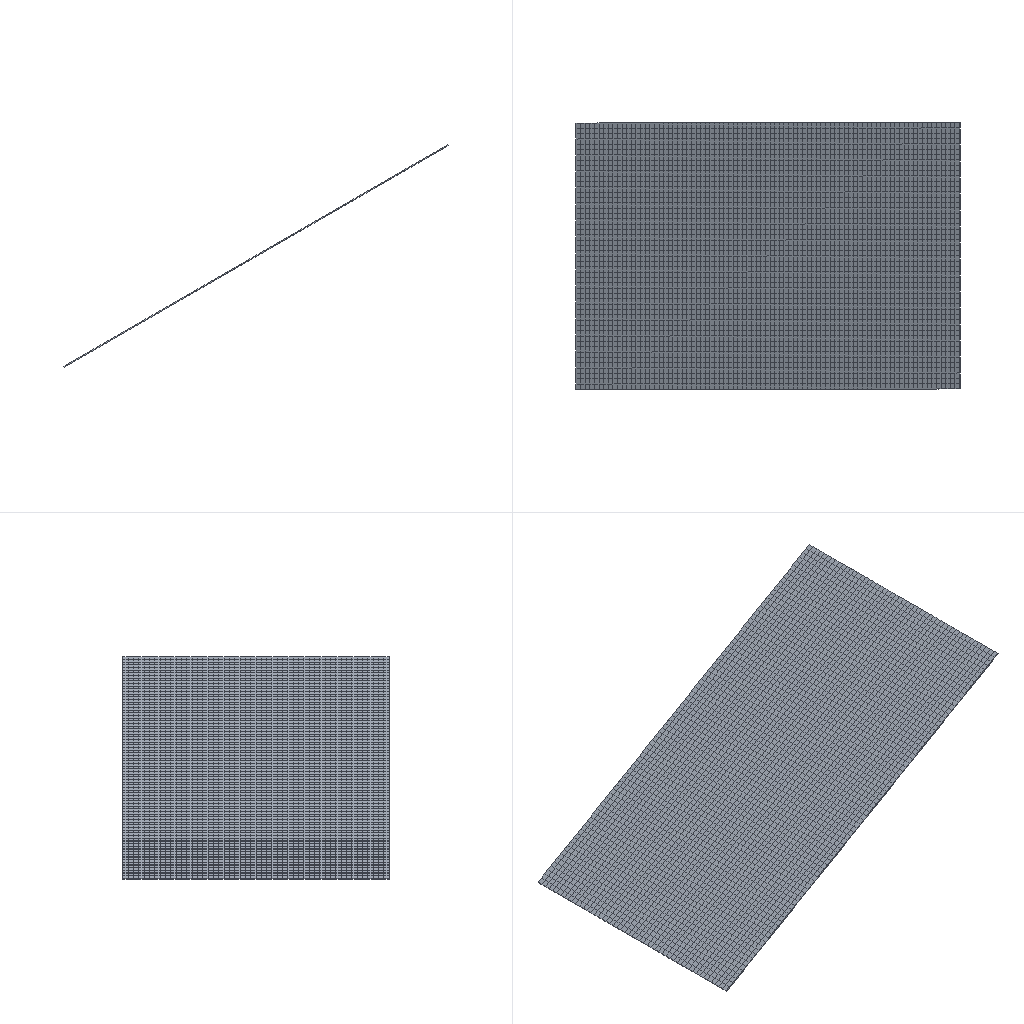Simulation study | abaqus
Set-up summary:
category,name,step,type,value,unit,region
solver,abaqus
solver,version,,,Abaqus/Standard 2020
units,not stated in the deck,,not stated
analysis,deck,,static,static
load_step,Step-1,Step-1,static
load_step,requested,,,1
mesh,nodes,,,21420
mesh,elements,,,16600
element_type,C3D8R,,solid,16600
load,load commands in deck,,count,1
bc,support commands in deck,,count,1
material,LAY1,,in results
material,LAY2,,in results
material,LAY4,,in results
check,setup vs results,,match,"per instance, exact: element labels, types and connectivity; labels of the nodes the elements use; coordinates of those nodes at SINGLE_PRECISION in 1 of 1 instance(s)"
Abaqus input file, long lists of numbers shortened:
*Heading
** Job name: Job-1 Model name: Model-1
** Generated by: Abaqus/CAE 2020
*Preprint, echo=NO, model=NO, history=NO, contact=NO
**
** PARTS
**
*Part, name=Part-1
*Node
      1,           0.,        -992.,  0.3
      2,           0.,           0.,  0.3
** (21418 more lines like these left out)
*Element, type=C3D8R
   1,  380, 1331, 5349,  217,    1,   21,  118,    4
   2, 1331, 1332, 5350, 5349,   21,   22,  117,  118
** (16598 more lines like these left out)
*Nset, nset=Set-1
    11,    12,    14,    15,    17,    18,    19,    20,   594,   595,   596,   597,   598,   599,   600,   601
   602,   603,   604,   605,   606,   607,   608,   609,   610,   611,   612,   613,   614,   615,   616,   617
** (534 more lines like these left out)
*Elset, elset=Set-1, generate
 12451,  16600,      1
*Nset, nset=Set-2
     1,     2,     5,     8,     9,    10,    11,    12,    13,    14,    15,    16,    21,    22,    23,    24
    25,    26,    27,    28,    29,    30,    31,    32,    33,    34,    35,    36,    37,    38,    39,    40
** (802 more lines like these left out)
*Elset, elset=Set-2, generate
  4151,  12450,      1
*Nset, nset=Set-3
    1,    2,    3,    4,    5,    6,    7,    8,   21,   22,   23,   24,   25,   26,   27,   28
   29,   30,   31,   32,   33,   34,   35,   36,   37,   38,   39,   40,   41,   42,   43,   44
** (534 more lines like these left out)
*Elset, elset=Set-3, generate
    1,  4150,     1
** Section: lay4
*Solid Section, elset=Set-3, material=lay4
,
** Section: lay2
*Solid Section, elset=Set-2, material=lay2
,
** Section: lay1
*Solid Section, elset=Set-1, material=lay1
,
*End Part
**
**
** ASSEMBLY
**
*Assembly, name=Assembly
**
*Instance, name=Part-1-1, part=Part-1
          0.,           0.,           0.
          0.,           0.,           0.,           0., -1.,           0., 30.
*End Instance
**
*Nset, nset=Set-1, instance=Part-1-1
    1,    2,    3,    4,    5,    6,    7,    8,    9,   10,   11,   12,   13,   14,   15,   16
   17,   18,   19,   20,   21,   22,   23,   24,   25,   26,   27,   28,   29,   30,   31,   32
** (30 more lines like these left out)
*Elset, elset=Set-1, instance=Part-1-1
     1,     2,     3,     4,     5,     6,     7,     8,     9,    10,    11,    12,    13,    14,    15,    16
    17,    18,    19,    20,    21,    22,    23,    24,    25,    26,    27,    28,    29,    30,    31,    32
** (23 more lines like these left out)
*Elset, elset=_Surf-1_S5, internal, instance=Part-1-1, generate
 12451,  16600,      1
*Surface, type=ELEMENT, name=Surf-1
_Surf-1_S5, S5
*End Assembly
*Amplitude, name=Amp-1
             0.,              0.,              1.,              1.
**
** MATERIALS
**
*Material, name=lay1
*Elastic
73000., 0.2
*Material, name=lay2
*Elastic
35., 0.15
*Material, name=lay4
*Elastic
2500., 0.43
** ----------------------------------------------------------------
**
** STEP: Step-1
**
*Step, name=Step-1, nlgeom=YES, inc=1000
*Static, stabilize=0.0002, allsdtol=0.05, continue=NO
0.01, 1., 1e-05, 1.
**
** BOUNDARY CONDITIONS
**
** Name: BC-1 Type: 对称/反对称/完全固定
*Boundary
Set-1, ENCASTRE
**
** LOADS
**
** Name: Load-1   Type: Surface traction
*Dsload, amplitude=Amp-1
Surf-1, TRVEC, 0.001, 1., 0., 0.
**
** OUTPUT REQUESTS
**
*Restart, write, frequency=0
**
** FIELD OUTPUT: F-Output-1
**
*Output, field, variable=PRESELECT
**
** HISTORY OUTPUT: H-Output-1
**
*Output, history, variable=PRESELECT
*End Step
Results summary:
result,step,,completed,increments=12 time=1.0/1.0
result,analysis,,,static
result,last_loadstep,,,1
result,primary field,,,U
result,reaction total,,FX,-1636.781,model units
result,reaction total,,FY,8e-06,model units
result,reaction total,,FZ,-0.001216,model units